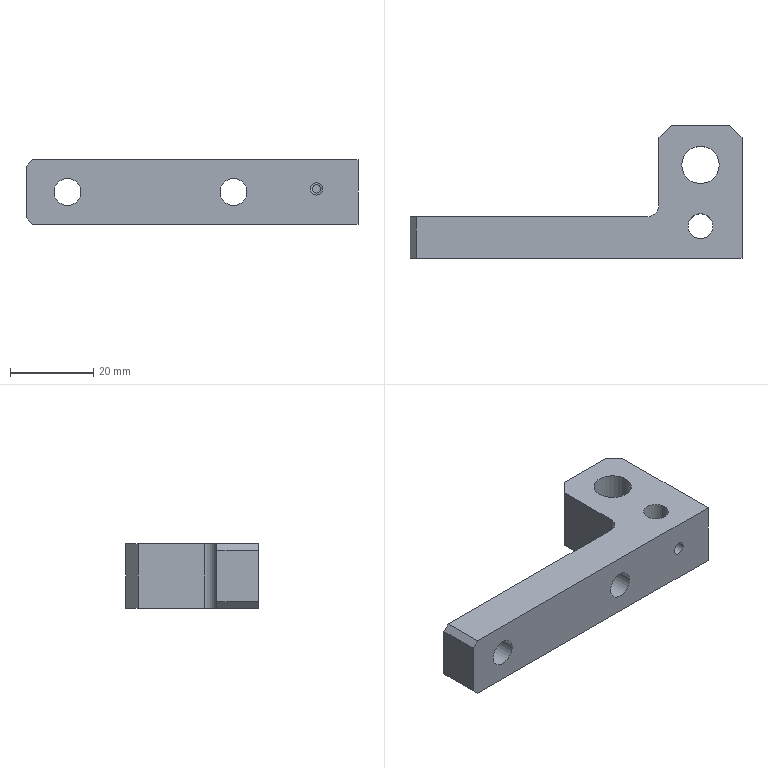NC program | NX | posted with a generic post | part box 80 x 32 x 15.5 mm
Lines 1193 to 2017 of 7013:
(PLANAR_MILL_4_COPY , TOOL : D5-15-D6-50-3T-ROUGH)
N2360 T04 M6
N2362 G53
N2364 G17 G0 G90 X28.923 Y-8.065 B0. C0. S3000 M3
N2366 G43 Z20. H4
N2368 Z-5.
N2370 G94 G1 X28.957 Y-8.092 Z-5.001 F400.
N2372 X29.143 Y-8.199 Z-5.007
N2374 X29.41 Y-8.309 Z-5.014
N2376 X29.692 Y-8.378 Z-5.022
N2378 X29.981 Y-8.403 Z-5.03
N2380 X30.27 Y-8.384 Z-5.037
N2382 X30.553 Y-8.321 Z-5.045
N2384 X30.823 Y-8.216 Z-5.052
N2386 X31.074 Y-8.071 Z-5.06
N2388 X31.3 Y-7.889 Z-5.067
N2390 X31.496 Y-7.676 Z-5.075
N2392 X31.658 Y-7.435 Z-5.083
N2394 X31.78 Y-7.172 Z-5.09
N2396 X31.862 Y-6.894 Z-5.098
N2398 X31.9 Y-6.607 Z-5.105
N2400 Y-6.393 Z-5.111
N2402 X31.862 Y-6.106 Z-5.119
N2404 X31.78 Y-5.828 Z-5.126
N2406 X31.658 Y-5.565 Z-5.134
N2408 X31.496 Y-5.324 Z-5.141
N2410 X31.3 Y-5.111 Z-5.149
N2412 X31.074 Y-4.929 Z-5.157
N2414 X30.823 Y-4.784 Z-5.164
N2416 X30.553 Y-4.679 Z-5.172
N2418 X30.27 Y-4.616 Z-5.179
N2420 X29.981 Y-4.597 Z-5.187
N2422 X29.692 Y-4.622 Z-5.195
N2424 X29.41 Y-4.691 Z-5.202
N2426 X29.143 Y-4.801 Z-5.21
N2428 X28.957 Y-4.908 Z-5.215
N2430 X28.723 Y-5.089 Z-5.223
N2432 X28.52 Y-5.304 Z-5.231
N2434 X28.352 Y-5.549 Z-5.239
N2436 X28.224 Y-5.816 Z-5.246
N2438 X28.14 Y-6.1 Z-5.254
N2440 X28.1 Y-6.393 Z-5.262
N2442 Y-6.607 Z-5.267
N2444 X28.14 Y-6.9 Z-5.275
N2446 X28.224 Y-7.184 Z-5.283
N2448 X28.352 Y-7.452 Z-5.291
N2450 X28.52 Y-7.696 Z-5.298
N2452 X28.723 Y-7.911 Z-5.306
N2454 X28.957 Y-8.092 Z-5.314
N2456 X29.143 Y-8.199 Z-5.32
N2458 X29.41 Y-8.309 Z-5.327
N2460 X29.692 Y-8.378 Z-5.335
N2462 X29.981 Y-8.403 Z-5.342
N2464 X30.27 Y-8.384 Z-5.35
N2466 X30.553 Y-8.321 Z-5.358
N2468 X30.823 Y-8.216 Z-5.365
N2470 X31.074 Y-8.071 Z-5.373
N2472 X31.3 Y-7.889 Z-5.38
N2474 X31.496 Y-7.676 Z-5.388
N2476 X31.658 Y-7.435 Z-5.395
N2478 X31.78 Y-7.172 Z-5.403
N2480 X31.862 Y-6.894 Z-5.411
N2482 X31.9 Y-6.607 Z-5.418
N2484 Y-6.393 Z-5.424
N2486 X31.862 Y-6.106 Z-5.431
N2488 X31.78 Y-5.828 Z-5.439
N2490 X31.658 Y-5.565 Z-5.447
N2492 X31.496 Y-5.324 Z-5.454
N2494 X31.3 Y-5.111 Z-5.462
N2496 X31.074 Y-4.929 Z-5.469
N2498 X30.823 Y-4.784 Z-5.477
N2500 X30.553 Y-4.679 Z-5.485
N2502 X30.27 Y-4.616 Z-5.492
N2504 X29.981 Y-4.597 Z-5.5
N2506 X29.692 Y-4.622 Z-5.507
N2508 X29.41 Y-4.691 Z-5.515
N2510 X29.143 Y-4.801 Z-5.522
N2512 X28.957 Y-4.908 Z-5.528
N2514 X28.723 Y-5.089 Z-5.536
N2516 X28.52 Y-5.304 Z-5.544
N2518 X28.352 Y-5.549 Z-5.551
N2520 X28.224 Y-5.816 Z-5.559
N2522 X28.14 Y-6.1 Z-5.567
N2524 X28.1 Y-6.393 Z-5.575
N2526 Y-6.607 Z-5.58
N2528 X28.14 Y-6.9 Z-5.588
N2530 X28.224 Y-7.184 Z-5.596
N2532 X28.352 Y-7.452 Z-5.603
N2534 X28.52 Y-7.696 Z-5.611
N2536 X28.723 Y-7.911 Z-5.619
N2538 X28.957 Y-8.092 Z-5.627
N2540 X29.143 Y-8.199 Z-5.632
N2542 X29.41 Y-8.309 Z-5.64
N2544 X29.692 Y-8.378 Z-5.648
N2546 X29.981 Y-8.403 Z-5.655
N2548 X30.27 Y-8.384 Z-5.663
N2550 X30.553 Y-8.321 Z-5.67
N2552 X30.823 Y-8.216 Z-5.678
N2554 X31.074 Y-8.071 Z-5.685
N2556 X31.3 Y-7.889 Z-5.693
N2558 X31.496 Y-7.676 Z-5.701
N2560 X31.658 Y-7.435 Z-5.708
N2562 X31.78 Y-7.172 Z-5.716
N2564 X31.862 Y-6.894 Z-5.723
N2566 X31.9 Y-6.607 Z-5.731
N2568 Y-6.393 Z-5.737
N2570 X31.862 Y-6.106 Z-5.744
N2572 X31.78 Y-5.828 Z-5.752
N2574 X31.658 Y-5.565 Z-5.759
N2576 X31.496 Y-5.324 Z-5.767
N2578 X31.3 Y-5.111 Z-5.775
N2580 X31.074 Y-4.929 Z-5.782
N2582 X30.823 Y-4.784 Z-5.79
N2584 X30.553 Y-4.679 Z-5.797
N2586 X30.27 Y-4.616 Z-5.805
N2588 X29.981 Y-4.597 Z-5.813
N2590 X29.692 Y-4.622 Z-5.82
N2592 X29.41 Y-4.691 Z-5.828
N2594 X29.143 Y-4.801 Z-5.835
N2596 X28.957 Y-4.908 Z-5.841
N2598 X28.723 Y-5.089 Z-5.849
N2600 X28.52 Y-5.304 Z-5.856
N2602 X28.352 Y-5.549 Z-5.864
N2604 X28.224 Y-5.816 Z-5.872
N2606 X28.14 Y-6.1 Z-5.88
N2608 X28.1 Y-6.393 Z-5.887
N2610 Y-6.607 Z-5.893
N2612 X28.14 Y-6.9 Z-5.901
N2614 X28.224 Y-7.184 Z-5.909
N2616 X28.352 Y-7.452 Z-5.916
N2618 X28.52 Y-7.696 Z-5.924
N2620 X28.723 Y-7.911 Z-5.932
N2622 X28.957 Y-8.092 Z-5.94
N2624 X29.143 Y-8.199 Z-5.945
N2626 X29.41 Y-8.309 Z-5.953
N2628 X29.692 Y-8.378 Z-5.96
N2630 X29.981 Y-8.403 Z-5.968
N2632 X30.27 Y-8.384 Z-5.976
N2634 X30.553 Y-8.321 Z-5.983
N2636 X30.823 Y-8.216 Z-5.991
N2638 X31.074 Y-8.071 Z-5.998
N2640 X31.3 Y-7.889 Z-6.006
N2642 X31.496 Y-7.676 Z-6.013
N2644 X31.658 Y-7.435 Z-6.021
N2646 X31.78 Y-7.172 Z-6.029
N2648 X31.862 Y-6.894 Z-6.036
N2650 X31.9 Y-6.607 Z-6.044
N2652 Y-6.393 Z-6.049
N2654 X31.862 Y-6.106 Z-6.057
N2656 X31.78 Y-5.828 Z-6.065
N2658 X31.658 Y-5.565 Z-6.072
N2660 X31.496 Y-5.324 Z-6.08
N2662 X31.3 Y-5.111 Z-6.087
N2664 X31.074 Y-4.929 Z-6.095
N2666 X30.823 Y-4.784 Z-6.103
N2668 X30.553 Y-4.679 Z-6.11
N2670 X30.27 Y-4.616 Z-6.118
N2672 X29.981 Y-4.597 Z-6.125
N2674 X29.692 Y-4.622 Z-6.133
N2676 X29.41 Y-4.691 Z-6.141
N2678 X29.143 Y-4.801 Z-6.148
N2680 X28.957 Y-4.908 Z-6.154
N2682 X28.723 Y-5.089 Z-6.161
N2684 X28.52 Y-5.304 Z-6.169
N2686 X28.352 Y-5.549 Z-6.177
N2688 X28.224 Y-5.816 Z-6.185
N2690 X28.14 Y-6.1 Z-6.192
N2692 X28.1 Y-6.393 Z-6.2
N2694 Y-6.607 Z-6.206
N2696 X28.14 Y-6.9 Z-6.214
N2698 X28.224 Y-7.184 Z-6.221
N2700 X28.352 Y-7.452 Z-6.229
N2702 X28.52 Y-7.696 Z-6.237
N2704 X28.723 Y-7.911 Z-6.245
N2706 X28.957 Y-8.092 Z-6.252
N2708 X29.143 Y-8.199 Z-6.258
N2710 X29.41 Y-8.309 Z-6.266
N2712 X29.692 Y-8.378 Z-6.273
N2714 X29.981 Y-8.403 Z-6.281
N2716 X30.27 Y-8.384 Z-6.288
N2718 X30.553 Y-8.321 Z-6.296
N2720 X30.823 Y-8.216 Z-6.304
N2722 X31.074 Y-8.071 Z-6.311
N2724 X31.3 Y-7.889 Z-6.319
N2726 X31.496 Y-7.676 Z-6.326
N2728 X31.658 Y-7.435 Z-6.334
N2730 X31.78 Y-7.172 Z-6.341
N2732 X31.862 Y-6.894 Z-6.349
N2734 X31.9 Y-6.607 Z-6.357
N2736 Y-6.393 Z-6.362
N2738 X31.862 Y-6.106 Z-6.37
N2740 X31.78 Y-5.828 Z-6.377
N2742 X31.658 Y-5.565 Z-6.385
N2744 X31.496 Y-5.324 Z-6.393
N2746 X31.3 Y-5.111 Z-6.4
N2748 X31.074 Y-4.929 Z-6.408
N2750 X30.823 Y-4.784 Z-6.415
N2752 X30.553 Y-4.679 Z-6.423
N2754 X30.27 Y-4.616 Z-6.431
N2756 X29.981 Y-4.597 Z-6.438
N2758 X29.692 Y-4.622 Z-6.446
N2760 X29.41 Y-4.691 Z-6.453
N2762 X29.143 Y-4.801 Z-6.461
N2764 X28.957 Y-4.908 Z-6.467
N2766 X28.723 Y-5.089 Z-6.474
N2768 X28.52 Y-5.304 Z-6.482
N2770 X28.352 Y-5.549 Z-6.49
N2772 X28.224 Y-5.816 Z-6.498
N2774 X28.14 Y-6.1 Z-6.505
N2776 X28.1 Y-6.393 Z-6.513
N2778 Y-6.607 Z-6.519
N2780 X28.14 Y-6.9 Z-6.526
N2782 X28.224 Y-7.184 Z-6.534
N2784 X28.352 Y-7.452 Z-6.542
N2786 X28.52 Y-7.696 Z-6.55
N2788 X28.723 Y-7.911 Z-6.557
N2790 X28.957 Y-8.092 Z-6.565
N2792 X29.143 Y-8.199 Z-6.571
N2794 X29.41 Y-8.309 Z-6.578
N2796 X29.692 Y-8.378 Z-6.586
N2798 X29.981 Y-8.403 Z-6.594
N2800 X30.27 Y-8.384 Z-6.601
N2802 X30.553 Y-8.321 Z-6.609
N2804 X30.823 Y-8.216 Z-6.616
N2806 X31.074 Y-8.071 Z-6.624
N2808 X31.3 Y-7.889 Z-6.631
N2810 X31.496 Y-7.676 Z-6.639
N2812 X31.658 Y-7.435 Z-6.647
N2814 X31.78 Y-7.172 Z-6.654
N2816 X31.862 Y-6.894 Z-6.662
N2818 X31.9 Y-6.607 Z-6.669
N2820 Y-6.393 Z-6.675
N2822 X31.862 Y-6.106 Z-6.683
N2824 X31.78 Y-5.828 Z-6.69
N2826 X31.658 Y-5.565 Z-6.698
N2828 X31.496 Y-5.324 Z-6.705
N2830 X31.3 Y-5.111 Z-6.713
N2832 X31.074 Y-4.929 Z-6.721
N2834 X30.823 Y-4.784 Z-6.728
N2836 X30.553 Y-4.679 Z-6.736
N2838 X30.27 Y-4.616 Z-6.743
N2840 X29.981 Y-4.597 Z-6.751
N2842 X29.692 Y-4.622 Z-6.759
N2844 X29.41 Y-4.691 Z-6.766
N2846 X29.143 Y-4.801 Z-6.774
N2848 X28.957 Y-4.908 Z-6.779
N2850 X28.723 Y-5.089 Z-6.787
N2852 X28.52 Y-5.304 Z-6.795
N2854 X28.352 Y-5.549 Z-6.803
N2856 X28.224 Y-5.816 Z-6.81
N2858 X28.14 Y-6.1 Z-6.818
N2860 X28.1 Y-6.393 Z-6.826
N2862 Y-6.607 Z-6.831
N2864 X28.14 Y-6.9 Z-6.839
N2866 X28.224 Y-7.184 Z-6.847
N2868 X28.352 Y-7.452 Z-6.855
N2870 X28.52 Y-7.696 Z-6.862
N2872 X28.723 Y-7.911 Z-6.87
N2874 X28.957 Y-8.092 Z-6.878
N2876 X29.143 Y-8.199 Z-6.884
N2878 X29.41 Y-8.309 Z-6.891
N2880 X29.692 Y-8.378 Z-6.899
N2882 X29.981 Y-8.403 Z-6.906
N2884 X30.27 Y-8.384 Z-6.914
N2886 X30.553 Y-8.321 Z-6.922
N2888 X30.823 Y-8.216 Z-6.929
N2890 X31.074 Y-8.071 Z-6.937
N2892 X31.3 Y-7.889 Z-6.944
N2894 X31.496 Y-7.676 Z-6.952
N2896 X31.658 Y-7.435 Z-6.959
N2898 X31.78 Y-7.172 Z-6.967
N2900 X31.862 Y-6.894 Z-6.975
N2902 X31.9 Y-6.607 Z-6.982
N2904 Y-6.393 Z-6.988
N2906 X31.862 Y-6.106 Z-6.995
N2908 X31.78 Y-5.828 Z-7.003
N2910 X31.658 Y-5.565 Z-7.011
N2912 X31.496 Y-5.324 Z-7.018
N2914 X31.3 Y-5.111 Z-7.026
N2916 X31.074 Y-4.929 Z-7.033
N2918 X30.823 Y-4.784 Z-7.041
N2920 X30.553 Y-4.679 Z-7.049
N2922 X30.27 Y-4.616 Z-7.056
N2924 X29.981 Y-4.597 Z-7.064
N2926 X29.692 Y-4.622 Z-7.071
N2928 X29.41 Y-4.691 Z-7.079
N2930 X29.143 Y-4.801 Z-7.087
N2932 X28.957 Y-4.908 Z-7.092
N2934 X28.723 Y-5.089 Z-7.1
N2936 X28.52 Y-5.304 Z-7.108
N2938 X28.352 Y-5.549 Z-7.115
N2940 X28.224 Y-5.816 Z-7.123
N2942 X28.14 Y-6.1 Z-7.131
N2944 X28.1 Y-6.393 Z-7.139
N2946 Y-6.607 Z-7.144
N2948 X28.14 Y-6.9 Z-7.152
N2950 X28.224 Y-7.184 Z-7.16
N2952 X28.352 Y-7.452 Z-7.168
N2954 X28.52 Y-7.696 Z-7.175
N2956 X28.723 Y-7.911 Z-7.183
N2958 X28.957 Y-8.092 Z-7.191
N2960 X29.143 Y-8.199 Z-7.196
N2962 X29.41 Y-8.309 Z-7.204
N2964 X29.692 Y-8.378 Z-7.212
N2966 X29.981 Y-8.403 Z-7.219
N2968 X30.27 Y-8.384 Z-7.227
N2970 X30.553 Y-8.321 Z-7.234
N2972 X30.823 Y-8.216 Z-7.242
N2974 X31.074 Y-8.071 Z-7.25
N2976 X31.3 Y-7.889 Z-7.257
N2978 X31.496 Y-7.676 Z-7.265
N2980 X31.658 Y-7.435 Z-7.272
N2982 X31.78 Y-7.172 Z-7.28
N2984 X31.862 Y-6.894 Z-7.287
N2986 X31.9 Y-6.607 Z-7.295
N2988 Y-6.393 Z-7.301
N2990 X31.862 Y-6.106 Z-7.308
N2992 X31.78 Y-5.828 Z-7.316
N2994 X31.658 Y-5.565 Z-7.323
N2996 X31.496 Y-5.324 Z-7.331
N2998 X31.3 Y-5.111 Z-7.339
N3000 X31.074 Y-4.929 Z-7.346
N3002 X30.823 Y-4.784 Z-7.354
N3004 X30.553 Y-4.679 Z-7.361
N3006 X30.27 Y-4.616 Z-7.369
N3008 X29.981 Y-4.597 Z-7.377
N3010 X29.692 Y-4.622 Z-7.384
N3012 X29.41 Y-4.691 Z-7.392
N3014 X29.143 Y-4.801 Z-7.399
N3016 X28.957 Y-4.908 Z-7.405
N3018 X28.723 Y-5.089 Z-7.413
N3020 X28.52 Y-5.304 Z-7.42
N3022 X28.352 Y-5.549 Z-7.428
N3024 X28.224 Y-5.816 Z-7.436
N3026 X28.14 Y-6.1 Z-7.444
N3028 X28.1 Y-6.393 Z-7.451
N3030 Y-6.607 Z-7.457
N3032 X28.14 Y-6.9 Z-7.465
N3034 X28.224 Y-7.184 Z-7.473
N3036 X28.352 Y-7.452 Z-7.48
N3038 X28.52 Y-7.696 Z-7.488
N3040 X28.723 Y-7.911 Z-7.496
N3042 X28.957 Y-8.092 Z-7.504
N3044 X29.143 Y-8.199 Z-7.509
N3046 X29.41 Y-8.309 Z-7.517
N3048 X29.692 Y-8.378 Z-7.524
N3050 X29.981 Y-8.403 Z-7.532
N3052 X30.27 Y-8.384 Z-7.54
N3054 X30.553 Y-8.321 Z-7.547
N3056 X30.823 Y-8.216 Z-7.555
N3058 X31.074 Y-8.071 Z-7.562
N3060 X31.3 Y-7.889 Z-7.57
N3062 X31.496 Y-7.676 Z-7.578
N3064 X31.658 Y-7.435 Z-7.585
N3066 X31.78 Y-7.172 Z-7.593
N3068 X31.862 Y-6.894 Z-7.6
N3070 X31.9 Y-6.607 Z-7.608
N3072 Y-6.393 Z-7.613
N3074 X31.862 Y-6.106 Z-7.621
N3076 X31.78 Y-5.828 Z-7.629
N3078 X31.658 Y-5.565 Z-7.636
N3080 X31.496 Y-5.324 Z-7.644
N3082 X31.3 Y-5.111 Z-7.651
N3084 X31.074 Y-4.929 Z-7.659
N3086 X30.823 Y-4.784 Z-7.667
N3088 X30.553 Y-4.679 Z-7.674
N3090 X30.27 Y-4.616 Z-7.682
N3092 X29.981 Y-4.597 Z-7.689
N3094 X29.692 Y-4.622 Z-7.697
N3096 X29.41 Y-4.691 Z-7.705
N3098 X29.143 Y-4.801 Z-7.712
N3100 X28.957 Y-4.908 Z-7.718
N3102 X28.723 Y-5.089 Z-7.725
N3104 X28.52 Y-5.304 Z-7.733
N3106 X28.352 Y-5.549 Z-7.741
N3108 X28.224 Y-5.816 Z-7.749
N3110 X28.14 Y-6.1 Z-7.757
N3112 X28.1 Y-6.393 Z-7.764
N3114 Y-6.607 Z-7.77
N3116 X28.14 Y-6.9 Z-7.778
N3118 X28.224 Y-7.184 Z-7.785
N3120 X28.352 Y-7.452 Z-7.793
N3122 X28.52 Y-7.696 Z-7.801
N3124 X28.723 Y-7.911 Z-7.809
N3126 X28.957 Y-8.092 Z-7.816
N3128 X29.143 Y-8.199 Z-7.822
N3130 X29.41 Y-8.309 Z-7.83
N3132 X29.692 Y-8.378 Z-7.837
N3134 X29.981 Y-8.403 Z-7.845
N3136 X30.27 Y-8.384 Z-7.852
N3138 X30.553 Y-8.321 Z-7.86
N3140 X30.823 Y-8.216 Z-7.868
N3142 X31.074 Y-8.071 Z-7.875
N3144 X31.3 Y-7.889 Z-7.883
N3146 X31.496 Y-7.676 Z-7.89
N3148 X31.658 Y-7.435 Z-7.898
N3150 X31.78 Y-7.172 Z-7.905
N3152 X31.862 Y-6.894 Z-7.913
N3154 X31.9 Y-6.607 Z-7.921
N3156 Y-6.393 Z-7.926
N3158 X31.862 Y-6.106 Z-7.934
N3160 X31.78 Y-5.828 Z-7.941
N3162 X31.658 Y-5.565 Z-7.949
N3164 X31.496 Y-5.324 Z-7.957
N3166 X31.3 Y-5.111 Z-7.964
N3168 X31.074 Y-4.929 Z-7.972
N3170 X30.823 Y-4.784 Z-7.979
N3172 X30.553 Y-4.679 Z-7.987
N3174 X30.27 Y-4.616 Z-7.995
N3176 X29.981 Y-4.597 Z-8.002
N3178 X29.692 Y-4.622 Z-8.01
N3180 X29.41 Y-4.691 Z-8.017
N3182 X29.143 Y-4.801 Z-8.025
N3184 X28.957 Y-4.908 Z-8.031
N3186 X28.723 Y-5.089 Z-8.038
N3188 X28.52 Y-5.304 Z-8.046
N3190 X28.352 Y-5.549 Z-8.054
N3192 X28.224 Y-5.816 Z-8.062
N3194 X28.14 Y-6.1 Z-8.069
N3196 X28.1 Y-6.393 Z-8.077
N3198 Y-6.607 Z-8.083
N3200 X28.14 Y-6.9 Z-8.09
N3202 X28.224 Y-7.184 Z-8.098
N3204 X28.352 Y-7.452 Z-8.106
N3206 X28.52 Y-7.696 Z-8.114
N3208 X28.723 Y-7.911 Z-8.121
N3210 X28.957 Y-8.092 Z-8.129
N3212 X29.143 Y-8.199 Z-8.135
N3214 X29.41 Y-8.309 Z-8.142
N3216 X29.692 Y-8.378 Z-8.15
N3218 X29.981 Y-8.403 Z-8.158
N3220 X30.27 Y-8.384 Z-8.165
N3222 X30.553 Y-8.321 Z-8.173
N3224 X30.823 Y-8.216 Z-8.18
N3226 X31.074 Y-8.071 Z-8.188
N3228 X31.3 Y-7.889 Z-8.196
N3230 X31.496 Y-7.676 Z-8.203
N3232 X31.658 Y-7.435 Z-8.211
N3234 X31.78 Y-7.172 Z-8.218
N3236 X31.862 Y-6.894 Z-8.226
N3238 X31.9 Y-6.607 Z-8.233
N3240 Y-6.393 Z-8.239
N3242 X31.862 Y-6.106 Z-8.247
N3244 X31.78 Y-5.828 Z-8.254
N3246 X31.658 Y-5.565 Z-8.262
N3248 X31.496 Y-5.324 Z-8.269
N3250 X31.3 Y-5.111 Z-8.277
N3252 X31.074 Y-4.929 Z-8.285
N3254 X30.823 Y-4.784 Z-8.292
N3256 X30.553 Y-4.679 Z-8.3
N3258 X30.27 Y-4.616 Z-8.307
N3260 X29.981 Y-4.597 Z-8.315
N3262 X29.692 Y-4.622 Z-8.323
N3264 X29.41 Y-4.691 Z-8.33
N3266 X29.143 Y-4.801 Z-8.338
N3268 X28.957 Y-4.908 Z-8.343
N3270 X28.723 Y-5.089 Z-8.351
N3272 X28.52 Y-5.304 Z-8.359
N3274 X28.352 Y-5.549 Z-8.367
N3276 X28.224 Y-5.816 Z-8.374
N3278 X28.14 Y-6.1 Z-8.382
N3280 X28.1 Y-6.393 Z-8.39
N3282 Y-6.607 Z-8.395
N3284 X28.14 Y-6.9 Z-8.403
N3286 X28.224 Y-7.184 Z-8.411
N3288 X28.352 Y-7.452 Z-8.419
N3290 X28.52 Y-7.696 Z-8.426
N3292 X28.723 Y-7.911 Z-8.434
N3294 X28.957 Y-8.092 Z-8.442
N3296 X29.143 Y-8.199 Z-8.448
N3298 X29.41 Y-8.309 Z-8.455
N3300 X29.692 Y-8.378 Z-8.463
N3302 X29.981 Y-8.403 Z-8.47
N3304 X30.27 Y-8.384 Z-8.478
N3306 X30.553 Y-8.321 Z-8.486
N3308 X30.823 Y-8.216 Z-8.493
N3310 X31.074 Y-8.071 Z-8.501
N3312 X31.3 Y-7.889 Z-8.508
N3314 X31.496 Y-7.676 Z-8.516
N3316 X31.658 Y-7.435 Z-8.524
N3318 X31.78 Y-7.172 Z-8.531
N3320 X31.862 Y-6.894 Z-8.539
N3322 X31.9 Y-6.607 Z-8.546
N3324 Y-6.393 Z-8.552
N3326 X31.862 Y-6.106 Z-8.559
N3328 X31.78 Y-5.828 Z-8.567
N3330 X31.658 Y-5.565 Z-8.575
N3332 X31.496 Y-5.324 Z-8.582
N3334 X31.3 Y-5.111 Z-8.59
N3336 X31.074 Y-4.929 Z-8.597
N3338 X30.823 Y-4.784 Z-8.605
N3340 X30.553 Y-4.679 Z-8.613
N3342 X30.27 Y-4.616 Z-8.62
N3344 X29.981 Y-4.597 Z-8.628
N3346 X29.692 Y-4.622 Z-8.635
N3348 X29.41 Y-4.691 Z-8.643
N3350 X29.143 Y-4.801 Z-8.651
N3352 X28.957 Y-4.908 Z-8.656
N3354 X28.723 Y-5.089 Z-8.664
N3356 X28.52 Y-5.304 Z-8.672
N3358 X28.352 Y-5.549 Z-8.679
N3360 X28.224 Y-5.816 Z-8.687
N3362 X28.14 Y-6.1 Z-8.695
N3364 X28.1 Y-6.393 Z-8.703
N3366 Y-6.607 Z-8.708
N3368 X28.14 Y-6.9 Z-8.716
N3370 X28.224 Y-7.184 Z-8.724
N3372 X28.352 Y-7.452 Z-8.732
N3374 X28.52 Y-7.696 Z-8.739
N3376 X28.723 Y-7.911 Z-8.747
N3378 X28.957 Y-8.092 Z-8.755
N3380 X29.143 Y-8.199 Z-8.76
N3382 X29.41 Y-8.309 Z-8.768
N3384 X29.692 Y-8.378 Z-8.776
N3386 X29.981 Y-8.403 Z-8.783
N3388 X30.27 Y-8.384 Z-8.791
N3390 X30.553 Y-8.321 Z-8.798
N3392 X30.823 Y-8.216 Z-8.806
N3394 X31.074 Y-8.071 Z-8.814
N3396 X31.3 Y-7.889 Z-8.821
N3398 X31.496 Y-7.676 Z-8.829
N3400 X31.658 Y-7.435 Z-8.836
N3402 X31.78 Y-7.172 Z-8.844
N3404 X31.862 Y-6.894 Z-8.851
N3406 X31.9 Y-6.607 Z-8.859
N3408 Y-6.393 Z-8.865
N3410 X31.862 Y-6.106 Z-8.872
N3412 X31.78 Y-5.828 Z-8.88
N3414 X31.658 Y-5.565 Z-8.887
N3416 X31.496 Y-5.324 Z-8.895
N3418 X31.3 Y-5.111 Z-8.903
N3420 X31.074 Y-4.929 Z-8.91
N3422 X30.823 Y-4.784 Z-8.918
N3424 X30.553 Y-4.679 Z-8.925
N3426 X30.27 Y-4.616 Z-8.933
N3428 X29.981 Y-4.597 Z-8.941
N3430 X29.692 Y-4.622 Z-8.948
N3432 X29.41 Y-4.691 Z-8.956
N3434 X29.143 Y-4.801 Z-8.963
N3436 X28.957 Y-4.908 Z-8.969
N3438 X28.723 Y-5.089 Z-8.977
N3440 X28.52 Y-5.304 Z-8.984
N3442 X28.352 Y-5.549 Z-8.992
N3444 X28.224 Y-5.816 Z-9.
N3446 X28.14 Y-6.1 Z-9.008
N3448 X28.1 Y-6.393 Z-9.015
N3450 Y-6.607 Z-9.021
N3452 X28.14 Y-6.9 Z-9.029
N3454 X28.224 Y-7.184 Z-9.037
N3456 X28.352 Y-7.452 Z-9.044
N3458 X28.52 Y-7.696 Z-9.052
N3460 X28.723 Y-7.911 Z-9.06
N3462 X28.957 Y-8.092 Z-9.068
N3464 X29.143 Y-8.199 Z-9.073
N3466 X29.41 Y-8.309 Z-9.081
N3468 X29.692 Y-8.378 Z-9.088
N3470 X29.981 Y-8.403 Z-9.096
N3472 X30.27 Y-8.384 Z-9.104
N3474 X30.553 Y-8.321 Z-9.111
N3476 X30.823 Y-8.216 Z-9.119
N3478 X31.074 Y-8.071 Z-9.126
N3480 X31.3 Y-7.889 Z-9.134
N3482 X31.496 Y-7.676 Z-9.142
N3484 X31.658 Y-7.435 Z-9.149
N3486 X31.78 Y-7.172 Z-9.157
N3488 X31.862 Y-6.894 Z-9.164
N3490 X31.9 Y-6.607 Z-9.172
N3492 Y-6.393 Z-9.177
N3494 X31.862 Y-6.106 Z-9.185
N3496 X31.78 Y-5.828 Z-9.193
N3498 X31.658 Y-5.565 Z-9.2
N3500 X31.496 Y-5.324 Z-9.208
N3502 X31.3 Y-5.111 Z-9.215
N3504 X31.074 Y-4.929 Z-9.223
N3506 X30.823 Y-4.784 Z-9.231
N3508 X30.553 Y-4.679 Z-9.238
N3510 X30.27 Y-4.616 Z-9.246
N3512 X29.981 Y-4.597 Z-9.253
N3514 X29.692 Y-4.622 Z-9.261
N3516 X29.41 Y-4.691 Z-9.269
N3518 X29.143 Y-4.801 Z-9.276
N3520 X28.957 Y-4.908 Z-9.282
N3522 X28.723 Y-5.089 Z-9.29
N3524 X28.52 Y-5.304 Z-9.297
N3526 X28.352 Y-5.549 Z-9.305
N3528 X28.224 Y-5.816 Z-9.313
N3530 X28.14 Y-6.1 Z-9.321
N3532 X28.1 Y-6.393 Z-9.328
N3534 Y-6.607 Z-9.334
N3536 X28.14 Y-6.9 Z-9.342
N3538 X28.224 Y-7.184 Z-9.349
N3540 X28.352 Y-7.452 Z-9.357
N3542 X28.52 Y-7.696 Z-9.365
N3544 X28.723 Y-7.911 Z-9.373
N3546 X28.957 Y-8.092 Z-9.38
N3548 X29.143 Y-8.199 Z-9.386
N3550 X29.41 Y-8.309 Z-9.394
N3552 X29.692 Y-8.378 Z-9.401
N3554 X29.981 Y-8.403 Z-9.409
N3556 X30.27 Y-8.384 Z-9.416
N3558 X30.553 Y-8.321 Z-9.424
N3560 X30.823 Y-8.216 Z-9.432
N3562 X31.074 Y-8.071 Z-9.439
N3564 X31.3 Y-7.889 Z-9.447
N3566 X31.496 Y-7.676 Z-9.454
N3568 X31.658 Y-7.435 Z-9.462
N3570 X31.78 Y-7.172 Z-9.47
N3572 X31.862 Y-6.894 Z-9.477
N3574 X31.9 Y-6.607 Z-9.485
N3576 Y-6.393 Z-9.49
N3578 X31.862 Y-6.106 Z-9.498
N3580 X31.78 Y-5.828 Z-9.505
N3582 X31.658 Y-5.565 Z-9.513
N3584 X31.496 Y-5.324 Z-9.521
N3586 X31.3 Y-5.111 Z-9.528
N3588 X31.074 Y-4.929 Z-9.536
N3590 X30.823 Y-4.784 Z-9.543
N3592 X30.553 Y-4.679 Z-9.551
N3594 X30.27 Y-4.616 Z-9.559
N3596 X29.981 Y-4.597 Z-9.566
N3598 X29.692 Y-4.622 Z-9.574
N3600 X29.41 Y-4.691 Z-9.581
N3602 X29.143 Y-4.801 Z-9.589
N3604 X28.957 Y-4.908 Z-9.595
N3606 X28.723 Y-5.089 Z-9.602
N3608 X28.52 Y-5.304 Z-9.61
N3610 X28.352 Y-5.549 Z-9.618
N3612 X28.224 Y-5.816 Z-9.626
N3614 X28.14 Y-6.1 Z-9.633
N3616 X28.1 Y-6.393 Z-9.641
N3618 Y-6.607 Z-9.647
N3620 X28.14 Y-6.9 Z-9.654
N3622 X28.224 Y-7.184 Z-9.662
N3624 X28.352 Y-7.452 Z-9.67
N3626 X28.52 Y-7.696 Z-9.678
N3628 X28.723 Y-7.911 Z-9.685
N3630 X28.957 Y-8.092 Z-9.693
N3632 X29.143 Y-8.199 Z-9.699
N3634 X29.41 Y-8.309 Z-9.706
N3636 X29.692 Y-8.378 Z-9.714
N3638 X29.981 Y-8.403 Z-9.722
N3640 X30.27 Y-8.384 Z-9.729
N3642 X30.553 Y-8.321 Z-9.737
N3644 X30.823 Y-8.216 Z-9.744
N3646 X31.074 Y-8.071 Z-9.752
N3648 X31.3 Y-7.889 Z-9.76
N3650 X31.496 Y-7.676 Z-9.767
N3652 X31.658 Y-7.435 Z-9.775
N3654 X31.78 Y-7.172 Z-9.782
N3656 X31.862 Y-6.894 Z-9.79
N3658 X31.9 Y-6.607 Z-9.798
N3660 Y-6.393 Z-9.803
N3662 X31.862 Y-6.106 Z-9.811
N3664 X31.78 Y-5.828 Z-9.818
N3666 X31.658 Y-5.565 Z-9.826
N3668 X31.496 Y-5.324 Z-9.833
N3670 X31.3 Y-5.111 Z-9.841
N3672 X31.074 Y-4.929 Z-9.849
N3674 X30.823 Y-4.784 Z-9.856
N3676 X30.553 Y-4.679 Z-9.864
N3678 X30.27 Y-4.616 Z-9.871
N3680 X29.981 Y-4.597 Z-9.879
N3682 X29.692 Y-4.622 Z-9.887
N3684 X29.41 Y-4.691 Z-9.894
N3686 X29.143 Y-4.801 Z-9.902
N3688 X28.957 Y-4.908 Z-9.907
N3690 X28.723 Y-5.089 Z-9.915
N3692 X28.52 Y-5.304 Z-9.923
N3694 X28.352 Y-5.549 Z-9.931
N3696 X28.224 Y-5.816 Z-9.938
N3698 X28.14 Y-6.1 Z-9.946
N3700 X28.1 Y-6.393 Z-9.954
N3702 Y-6.607 Z-9.959
N3704 X28.14 Y-6.9 Z-9.967
N3706 X28.224 Y-7.184 Z-9.975
N3708 X28.352 Y-7.452 Z-9.983
N3710 X28.52 Y-7.696 Z-9.991
N3712 X28.723 Y-7.911 Z-9.998
N3714 X28.957 Y-8.092 Z-10.006
N3716 X29.143 Y-8.199 Z-10.012
N3718 X29.41 Y-8.309 Z-10.019
N3720 X29.692 Y-8.378 Z-10.027
N3722 X29.981 Y-8.403 Z-10.034
N3724 X30.27 Y-8.384 Z-10.042
N3726 X30.553 Y-8.321 Z-10.05
N3728 X30.823 Y-8.216 Z-10.057
N3730 X31.074 Y-8.071 Z-10.065
N3732 X31.3 Y-7.889 Z-10.072
N3734 X31.496 Y-7.676 Z-10.08
N3736 X31.658 Y-7.435 Z-10.088
N3738 X31.78 Y-7.172 Z-10.095
N3740 X31.862 Y-6.894 Z-10.103
N3742 X31.9 Y-6.607 Z-10.11
N3744 Y-6.393 Z-10.116
N3746 X31.862 Y-6.106 Z-10.123
N3748 X31.78 Y-5.828 Z-10.131
N3750 X31.658 Y-5.565 Z-10.139
N3752 X31.496 Y-5.324 Z-10.146
N3754 X31.3 Y-5.111 Z-10.154
N3756 X31.074 Y-4.929 Z-10.161
N3758 X30.823 Y-4.784 Z-10.169
N3760 X30.553 Y-4.679 Z-10.177
N3762 X30.27 Y-4.616 Z-10.184
N3764 X29.981 Y-4.597 Z-10.192
N3766 X29.692 Y-4.622 Z-10.199
N3768 X29.41 Y-4.691 Z-10.207
N3770 X29.143 Y-4.801 Z-10.215
N3772 X28.957 Y-4.908 Z-10.22
N3774 X28.723 Y-5.089 Z-10.228
N3776 X28.52 Y-5.304 Z-10.236
N3778 X28.352 Y-5.549 Z-10.243
N3780 X28.224 Y-5.816 Z-10.251
N3782 X28.14 Y-6.1 Z-10.259
N3784 X28.1 Y-6.393 Z-10.267
N3786 Y-6.607 Z-10.272
N3788 X28.14 Y-6.9 Z-10.28
N3790 X28.224 Y-7.184 Z-10.288
N3792 X28.352 Y-7.452 Z-10.296
N3794 X28.52 Y-7.696 Z-10.303
N3796 X28.723 Y-7.911 Z-10.311
N3798 X28.957 Y-8.092 Z-10.319
N3800 X29.143 Y-8.199 Z-10.324
N3802 X29.41 Y-8.309 Z-10.332
N3804 X29.692 Y-8.378 Z-10.34
N3806 X29.981 Y-8.403 Z-10.347
N3808 X30.27 Y-8.384 Z-10.355
N3810 X30.553 Y-8.321 Z-10.362
N3812 X30.823 Y-8.216 Z-10.37
N3814 X31.074 Y-8.071 Z-10.378
N3816 X31.3 Y-7.889 Z-10.385
N3818 X31.496 Y-7.676 Z-10.393
N3820 X31.658 Y-7.435 Z-10.4
N3822 X31.78 Y-7.172 Z-10.408
N3824 X31.862 Y-6.894 Z-10.416
N3826 X31.9 Y-6.607 Z-10.423
N3828 Y-6.393 Z-10.429
N3830 X31.862 Y-6.106 Z-10.436
N3832 X31.78 Y-5.828 Z-10.444
N3834 X31.658 Y-5.565 Z-10.451
N3836 X31.496 Y-5.324 Z-10.459
N3838 X31.3 Y-5.111 Z-10.467
N3840 X31.074 Y-4.929 Z-10.474
N3842 X30.823 Y-4.784 Z-10.482
N3844 X30.553 Y-4.679 Z-10.489
N3846 X30.27 Y-4.616 Z-10.497
N3848 X29.981 Y-4.597 Z-10.505
N3850 X29.692 Y-4.622 Z-10.512
N3852 X29.41 Y-4.691 Z-10.52
N3854 X29.143 Y-4.801 Z-10.527
N3856 X28.957 Y-4.908 Z-10.533
N3858 X28.723 Y-5.089 Z-10.541
N3860 X28.52 Y-5.304 Z-10.548
N3862 X28.352 Y-5.549 Z-10.556
N3864 X28.224 Y-5.816 Z-10.564
N3866 X28.14 Y-6.1 Z-10.572
N3868 X28.1 Y-6.393 Z-10.58
N3870 Y-6.607 Z-10.585
N3872 X28.14 Y-6.9 Z-10.593
N3874 X28.224 Y-7.184 Z-10.601
N3876 X28.352 Y-7.452 Z-10.608
N3878 X28.52 Y-7.696 Z-10.616
N3880 X28.723 Y-7.911 Z-10.624
N3882 X28.957 Y-8.092 Z-10.632
N3884 X29.143 Y-8.199 Z-10.637
N3886 X29.41 Y-8.309 Z-10.645
N3888 X29.692 Y-8.378 Z-10.652
N3890 X29.981 Y-8.403 Z-10.66
N3892 X30.27 Y-8.384 Z-10.668
N3894 X30.553 Y-8.321 Z-10.675
N3896 X30.823 Y-8.216 Z-10.683
N3898 X31.074 Y-8.071 Z-10.69
N3900 X31.3 Y-7.889 Z-10.698
N3902 X31.496 Y-7.676 Z-10.706
N3904 X31.658 Y-7.435 Z-10.713
N3906 X31.78 Y-7.172 Z-10.721
N3908 X31.862 Y-6.894 Z-10.728
N3910 X31.9 Y-6.607 Z-10.736
N3912 Y-6.393 Z-10.742
N3914 X31.862 Y-6.106 Z-10.749
N3916 X31.78 Y-5.828 Z-10.757
N3918 X31.658 Y-5.565 Z-10.764
N3920 X31.496 Y-5.324 Z-10.772
N3922 X31.3 Y-5.111 Z-10.779
N3924 X31.074 Y-4.929 Z-10.787
N3926 X30.823 Y-4.784 Z-10.795
N3928 X30.553 Y-4.679 Z-10.802
N3930 X30.27 Y-4.616 Z-10.81
N3932 X29.981 Y-4.597 Z-10.817
N3934 X29.692 Y-4.622 Z-10.825
N3936 X29.41 Y-4.691 Z-10.833
N3938 X29.143 Y-4.801 Z-10.84
N3940 X28.957 Y-4.908 Z-10.846
N3942 X28.723 Y-5.089 Z-10.854
N3944 X28.52 Y-5.304 Z-10.861
N3946 X28.352 Y-5.549 Z-10.869
N3948 X28.224 Y-5.816 Z-10.877
N3950 X28.14 Y-6.1 Z-10.885
N3952 X28.1 Y-6.393 Z-10.892
N3954 Y-6.607 Z-10.898
N3956 X28.14 Y-6.9 Z-10.906
N3958 X28.224 Y-7.184 Z-10.913
N3960 X28.352 Y-7.452 Z-10.921
N3962 X28.52 Y-7.696 Z-10.929
N3964 X28.723 Y-7.911 Z-10.937
N3966 X28.957 Y-8.092 Z-10.944
N3968 X29.143 Y-8.199 Z-10.95
N3970 X29.41 Y-8.309 Z-10.958
N3972 X29.692 Y-8.378 Z-10.965
N3974 X29.981 Y-8.403 Z-10.973
N3976 X30.27 Y-8.384 Z-10.98
N3978 X30.553 Y-8.321 Z-10.988
N3980 X30.823 Y-8.216 Z-10.996
N3982 X31.074 Y-8.071 Z-11.003
N3984 X31.3 Y-7.889 Z-11.011
N3986 X31.496 Y-7.676 Z-11.018
N3988 X31.658 Y-7.435 Z-11.026
N3990 X31.78 Y-7.172 Z-11.034
N3992 X31.862 Y-6.894 Z-11.041
N3994 X31.9 Y-6.607 Z-11.049
N3996 Y-6.393 Z-11.054
N3998 X31.862 Y-6.106 Z-11.062
N4000 X31.78 Y-5.828 Z-11.069
N4002 X31.658 Y-5.565 Z-11.077